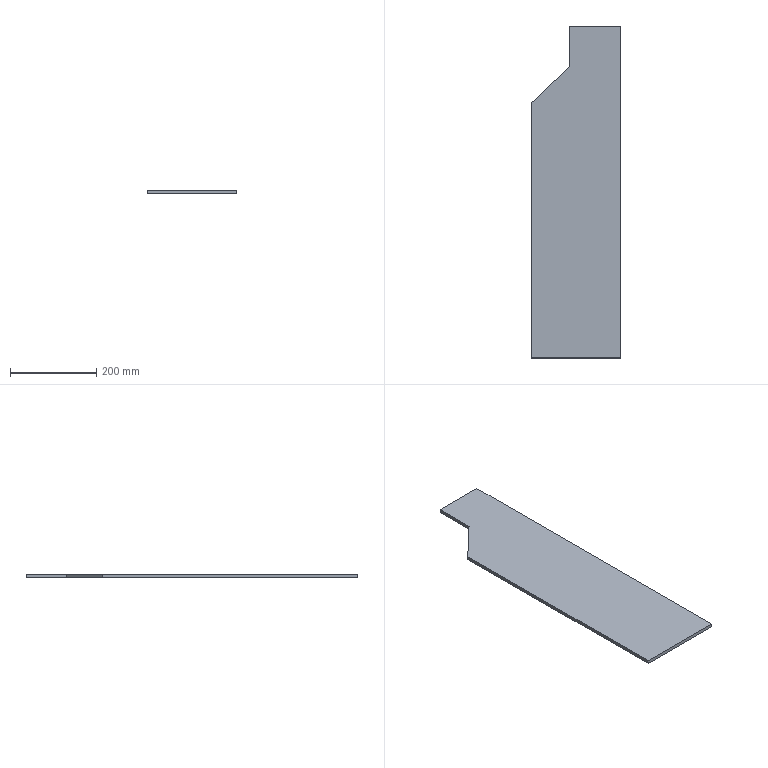Part | STEP file | Part 8 | 1 solid | 8 faces | box 208 x 768 x 8 mm | volume 1182208 mm3 | plane 8
STEP:
#1=CARTESIAN_POINT('',(0.,0.,0.));
#2=DIRECTION('',(0.,0.,1.));
#3=DIRECTION('',(1.,0.,0.));
#4=AXIS2_PLACEMENT_3D('',#1,#2,#3);
#5=CARTESIAN_POINT('',(0.,-384.,0.));
#6=VERTEX_POINT('',#5);
#7=CARTESIAN_POINT('',(0.,384.,0.));
#8=VERTEX_POINT('',#7);
#9=CARTESIAN_POINT('',(0.,-384.,0.));
#10=DIRECTION('',(0.,1.,0.));
#11=VECTOR('',#10,1.);
#12=LINE('',#9,#11);
#13=CARTESIAN_POINT('',(0.,-384.,8.));
#14=DIRECTION('',(-1.,0.,0.));
#15=DIRECTION('',(0.,0.,1.));
#16=AXIS2_PLACEMENT_3D('',#13,#14,#15);
#17=PLANE('',#16);
#18=CARTESIAN_POINT('',(-8.,0.));
#19=DIRECTION('',(0.,1.));
#20=VECTOR('',#19,1.);
#21=LINE('',#18,#20);
#22=(GEOMETRIC_REPRESENTATION_CONTEXT(2)PARAMETRIC_REPRESENTATION_CONTEXT()REPRESENTATION_CONTEXT('',''));
#23=DEFINITIONAL_REPRESENTATION('',(#21),#22);
#24=PCURVE('',#17,#23);
#25=CARTESIAN_POINT('',(0.,0.,0.));
#26=DIRECTION('',(0.,0.,-1.));
#27=DIRECTION('',(-1.,0.,0.));
#28=AXIS2_PLACEMENT_3D('',#25,#26,#27);
#29=PLANE('',#28);
#30=CARTESIAN_POINT('',(0.,-384.));
#31=DIRECTION('',(0.,1.));
#32=VECTOR('',#31,1.);
#33=LINE('',#30,#32);
#34=(GEOMETRIC_REPRESENTATION_CONTEXT(2)PARAMETRIC_REPRESENTATION_CONTEXT()REPRESENTATION_CONTEXT('',''));
#35=DEFINITIONAL_REPRESENTATION('',(#33),#34);
#36=PCURVE('',#29,#35);
#37=SURFACE_CURVE('',#12,(#24,#36),.PCURVE_S1.);
#38=EDGE_CURVE('',#6,#8,#37,.T.);
#39=ORIENTED_EDGE('',*,*,#38,.T.);
#40=CARTESIAN_POINT('',(0.,384.,8.));
#41=VERTEX_POINT('',#40);
#42=CARTESIAN_POINT('',(0.,384.,8.));
#43=DIRECTION('',(0.,0.,-1.));
#44=VECTOR('',#43,1.);
#45=LINE('',#42,#44);
#46=CARTESIAN_POINT('',(0.,768.));
#47=DIRECTION('',(-1.,0.));
#48=VECTOR('',#47,1.);
#49=LINE('',#46,#48);
#50=(GEOMETRIC_REPRESENTATION_CONTEXT(2)PARAMETRIC_REPRESENTATION_CONTEXT()REPRESENTATION_CONTEXT('',''));
#51=DEFINITIONAL_REPRESENTATION('',(#49),#50);
#52=PCURVE('',#17,#51);
#53=CARTESIAN_POINT('',(-120.,384.,8.));
#54=DIRECTION('',(0.,-1.,0.));
#55=DIRECTION('',(0.,0.,-1.));
#56=AXIS2_PLACEMENT_3D('',#53,#54,#55);
#57=PLANE('',#56);
#58=CARTESIAN_POINT('',(0.,120.));
#59=DIRECTION('',(1.,0.));
#60=VECTOR('',#59,1.);
#61=LINE('',#58,#60);
#62=(GEOMETRIC_REPRESENTATION_CONTEXT(2)PARAMETRIC_REPRESENTATION_CONTEXT()REPRESENTATION_CONTEXT('',''));
#63=DEFINITIONAL_REPRESENTATION('',(#61),#62);
#64=PCURVE('',#57,#63);
#65=SURFACE_CURVE('',#45,(#52,#64),.PCURVE_S1.);
#66=EDGE_CURVE('',#41,#8,#65,.T.);
#67=ORIENTED_EDGE('',*,*,#66,.F.);
#68=CARTESIAN_POINT('',(0.,-384.,8.));
#69=VERTEX_POINT('',#68);
#70=CARTESIAN_POINT('',(0.,-384.,8.));
#71=DIRECTION('',(0.,1.,0.));
#72=VECTOR('',#71,1.);
#73=LINE('',#70,#72);
#74=CARTESIAN_POINT('',(0.,0.));
#75=DIRECTION('',(0.,1.));
#76=VECTOR('',#75,1.);
#77=LINE('',#74,#76);
#78=(GEOMETRIC_REPRESENTATION_CONTEXT(2)PARAMETRIC_REPRESENTATION_CONTEXT()REPRESENTATION_CONTEXT('',''));
#79=DEFINITIONAL_REPRESENTATION('',(#77),#78);
#80=PCURVE('',#17,#79);
#81=CARTESIAN_POINT('',(0.,0.,8.));
#82=DIRECTION('',(0.,0.,-1.));
#83=DIRECTION('',(-1.,0.,0.));
#84=AXIS2_PLACEMENT_3D('',#81,#82,#83);
#85=PLANE('',#84);
#86=CARTESIAN_POINT('',(0.,-384.));
#87=DIRECTION('',(0.,1.));
#88=VECTOR('',#87,1.);
#89=LINE('',#86,#88);
#90=(GEOMETRIC_REPRESENTATION_CONTEXT(2)PARAMETRIC_REPRESENTATION_CONTEXT()REPRESENTATION_CONTEXT('',''));
#91=DEFINITIONAL_REPRESENTATION('',(#89),#90);
#92=PCURVE('',#85,#91);
#93=SURFACE_CURVE('',#73,(#80,#92),.PCURVE_S1.);
#94=EDGE_CURVE('',#69,#41,#93,.T.);
#95=ORIENTED_EDGE('',*,*,#94,.F.);
#96=CARTESIAN_POINT('',(0.,-384.,8.));
#97=DIRECTION('',(0.,0.,-1.));
#98=VECTOR('',#97,1.);
#99=LINE('',#96,#98);
#100=CARTESIAN_POINT('',(0.,0.));
#101=DIRECTION('',(-1.,0.));
#102=VECTOR('',#101,1.);
#103=LINE('',#100,#102);
#104=(GEOMETRIC_REPRESENTATION_CONTEXT(2)PARAMETRIC_REPRESENTATION_CONTEXT()REPRESENTATION_CONTEXT('',''));
#105=DEFINITIONAL_REPRESENTATION('',(#103),#104);
#106=PCURVE('',#17,#105);
#107=CARTESIAN_POINT('',(0.,-384.,8.));
#108=DIRECTION('',(0.,1.,0.));
#109=DIRECTION('',(0.,0.,1.));
#110=AXIS2_PLACEMENT_3D('',#107,#108,#109);
#111=PLANE('',#110);
#112=CARTESIAN_POINT('',(0.,0.));
#113=DIRECTION('',(-1.,0.));
#114=VECTOR('',#113,1.);
#115=LINE('',#112,#114);
#116=(GEOMETRIC_REPRESENTATION_CONTEXT(2)PARAMETRIC_REPRESENTATION_CONTEXT()REPRESENTATION_CONTEXT('',''));
#117=DEFINITIONAL_REPRESENTATION('',(#115),#116);
#118=PCURVE('',#111,#117);
#119=SURFACE_CURVE('',#99,(#106,#118),.PCURVE_S1.);
#120=EDGE_CURVE('',#69,#6,#119,.T.);
#121=ORIENTED_EDGE('',*,*,#120,.T.);
#122=EDGE_LOOP('',(#39,#67,#95,#121));
#123=FACE_BOUND('',#122,.T.);
#124=ADVANCED_FACE('',(#123),#17,.F.);
#125=CARTESIAN_POINT('',(-120.,384.,0.));
#126=VERTEX_POINT('',#125);
#127=CARTESIAN_POINT('',(-120.,384.,0.));
#128=DIRECTION('',(-1.,0.,0.));
#129=VECTOR('',#128,1.);
#130=LINE('',#127,#129);
#131=CARTESIAN_POINT('',(8.,0.));
#132=DIRECTION('',(0.,-1.));
#133=VECTOR('',#132,1.);
#134=LINE('',#131,#133);
#135=(GEOMETRIC_REPRESENTATION_CONTEXT(2)PARAMETRIC_REPRESENTATION_CONTEXT()REPRESENTATION_CONTEXT('',''));
#136=DEFINITIONAL_REPRESENTATION('',(#134),#135);
#137=PCURVE('',#57,#136);
#138=CARTESIAN_POINT('',(120.,384.));
#139=DIRECTION('',(1.,0.));
#140=VECTOR('',#139,1.);
#141=LINE('',#138,#140);
#142=(GEOMETRIC_REPRESENTATION_CONTEXT(2)PARAMETRIC_REPRESENTATION_CONTEXT()REPRESENTATION_CONTEXT('',''));
#143=DEFINITIONAL_REPRESENTATION('',(#141),#142);
#144=PCURVE('',#29,#143);
#145=SURFACE_CURVE('',#130,(#137,#144),.PCURVE_S1.);
#146=EDGE_CURVE('',#8,#126,#145,.T.);
#147=ORIENTED_EDGE('',*,*,#146,.T.);
#148=CARTESIAN_POINT('',(-120.,384.,8.));
#149=VERTEX_POINT('',#148);
#150=CARTESIAN_POINT('',(-120.,384.,8.));
#151=DIRECTION('',(0.,0.,-1.));
#152=VECTOR('',#151,1.);
#153=LINE('',#150,#152);
#154=CARTESIAN_POINT('',(0.,0.));
#155=DIRECTION('',(1.,0.));
#156=VECTOR('',#155,1.);
#157=LINE('',#154,#156);
#158=(GEOMETRIC_REPRESENTATION_CONTEXT(2)PARAMETRIC_REPRESENTATION_CONTEXT()REPRESENTATION_CONTEXT('',''));
#159=DEFINITIONAL_REPRESENTATION('',(#157),#158);
#160=PCURVE('',#57,#159);
#161=CARTESIAN_POINT('',(-120.,290.,8.));
#162=DIRECTION('',(1.,0.,0.));
#163=DIRECTION('',(0.,1.,0.));
#164=AXIS2_PLACEMENT_3D('',#161,#162,#163);
#165=PLANE('',#164);
#166=CARTESIAN_POINT('',(94.,0.));
#167=DIRECTION('',(0.,-1.));
#168=VECTOR('',#167,1.);
#169=LINE('',#166,#168);
#170=(GEOMETRIC_REPRESENTATION_CONTEXT(2)PARAMETRIC_REPRESENTATION_CONTEXT()REPRESENTATION_CONTEXT('',''));
#171=DEFINITIONAL_REPRESENTATION('',(#169),#170);
#172=PCURVE('',#165,#171);
#173=SURFACE_CURVE('',#153,(#160,#172),.PCURVE_S1.);
#174=EDGE_CURVE('',#149,#126,#173,.T.);
#175=ORIENTED_EDGE('',*,*,#174,.F.);
#176=CARTESIAN_POINT('',(-120.,384.,8.));
#177=DIRECTION('',(-1.,0.,0.));
#178=VECTOR('',#177,1.);
#179=LINE('',#176,#178);
#180=CARTESIAN_POINT('',(0.,0.));
#181=DIRECTION('',(0.,-1.));
#182=VECTOR('',#181,1.);
#183=LINE('',#180,#182);
#184=(GEOMETRIC_REPRESENTATION_CONTEXT(2)PARAMETRIC_REPRESENTATION_CONTEXT()REPRESENTATION_CONTEXT('',''));
#185=DEFINITIONAL_REPRESENTATION('',(#183),#184);
#186=PCURVE('',#57,#185);
#187=CARTESIAN_POINT('',(120.,384.));
#188=DIRECTION('',(1.,0.));
#189=VECTOR('',#188,1.);
#190=LINE('',#187,#189);
#191=(GEOMETRIC_REPRESENTATION_CONTEXT(2)PARAMETRIC_REPRESENTATION_CONTEXT()REPRESENTATION_CONTEXT('',''));
#192=DEFINITIONAL_REPRESENTATION('',(#190),#191);
#193=PCURVE('',#85,#192);
#194=SURFACE_CURVE('',#179,(#186,#193),.PCURVE_S1.);
#195=EDGE_CURVE('',#41,#149,#194,.T.);
#196=ORIENTED_EDGE('',*,*,#195,.F.);
#197=ORIENTED_EDGE('',*,*,#66,.T.);
#198=EDGE_LOOP('',(#147,#175,#196,#197));
#199=FACE_BOUND('',#198,.T.);
#200=ADVANCED_FACE('',(#199),#57,.F.);
#201=CARTESIAN_POINT('',(-120.,290.,0.));
#202=VERTEX_POINT('',#201);
#203=CARTESIAN_POINT('',(-120.,290.,0.));
#204=DIRECTION('',(0.,-1.,0.));
#205=VECTOR('',#204,1.);
#206=LINE('',#203,#205);
#207=CARTESIAN_POINT('',(0.,-8.));
#208=DIRECTION('',(-1.,0.));
#209=VECTOR('',#208,1.);
#210=LINE('',#207,#209);
#211=(GEOMETRIC_REPRESENTATION_CONTEXT(2)PARAMETRIC_REPRESENTATION_CONTEXT()REPRESENTATION_CONTEXT('',''));
#212=DEFINITIONAL_REPRESENTATION('',(#210),#211);
#213=PCURVE('',#165,#212);
#214=CARTESIAN_POINT('',(120.,290.));
#215=DIRECTION('',(0.,-1.));
#216=VECTOR('',#215,1.);
#217=LINE('',#214,#216);
#218=(GEOMETRIC_REPRESENTATION_CONTEXT(2)PARAMETRIC_REPRESENTATION_CONTEXT()REPRESENTATION_CONTEXT('',''));
#219=DEFINITIONAL_REPRESENTATION('',(#217),#218);
#220=PCURVE('',#29,#219);
#221=SURFACE_CURVE('',#206,(#213,#220),.PCURVE_S1.);
#222=EDGE_CURVE('',#126,#202,#221,.T.);
#223=ORIENTED_EDGE('',*,*,#222,.T.);
#224=CARTESIAN_POINT('',(-120.,290.,8.));
#225=VERTEX_POINT('',#224);
#226=CARTESIAN_POINT('',(-120.,290.,8.));
#227=DIRECTION('',(0.,0.,-1.));
#228=VECTOR('',#227,1.);
#229=LINE('',#226,#228);
#230=CARTESIAN_POINT('',(0.,0.));
#231=DIRECTION('',(0.,-1.));
#232=VECTOR('',#231,1.);
#233=LINE('',#230,#232);
#234=(GEOMETRIC_REPRESENTATION_CONTEXT(2)PARAMETRIC_REPRESENTATION_CONTEXT()REPRESENTATION_CONTEXT('',''));
#235=DEFINITIONAL_REPRESENTATION('',(#233),#234);
#236=PCURVE('',#165,#235);
#237=CARTESIAN_POINT('',(-208.,206.,8.));
#238=DIRECTION('',(0.6905,-0.7234,0.));
#239=DIRECTION('',(0.7234,0.6905,0.));
#240=AXIS2_PLACEMENT_3D('',#237,#238,#239);
#241=PLANE('',#240);
#242=CARTESIAN_POINT('',(121.655,0.));
#243=DIRECTION('',(0.,-1.));
#244=VECTOR('',#243,1.);
#245=LINE('',#242,#244);
#246=(GEOMETRIC_REPRESENTATION_CONTEXT(2)PARAMETRIC_REPRESENTATION_CONTEXT()REPRESENTATION_CONTEXT('',''));
#247=DEFINITIONAL_REPRESENTATION('',(#245),#246);
#248=PCURVE('',#241,#247);
#249=SURFACE_CURVE('',#229,(#236,#248),.PCURVE_S1.);
#250=EDGE_CURVE('',#225,#202,#249,.T.);
#251=ORIENTED_EDGE('',*,*,#250,.F.);
#252=CARTESIAN_POINT('',(-120.,290.,8.));
#253=DIRECTION('',(0.,-1.,0.));
#254=VECTOR('',#253,1.);
#255=LINE('',#252,#254);
#256=CARTESIAN_POINT('',(0.,0.));
#257=DIRECTION('',(-1.,0.));
#258=VECTOR('',#257,1.);
#259=LINE('',#256,#258);
#260=(GEOMETRIC_REPRESENTATION_CONTEXT(2)PARAMETRIC_REPRESENTATION_CONTEXT()REPRESENTATION_CONTEXT('',''));
#261=DEFINITIONAL_REPRESENTATION('',(#259),#260);
#262=PCURVE('',#165,#261);
#263=CARTESIAN_POINT('',(120.,290.));
#264=DIRECTION('',(0.,-1.));
#265=VECTOR('',#264,1.);
#266=LINE('',#263,#265);
#267=(GEOMETRIC_REPRESENTATION_CONTEXT(2)PARAMETRIC_REPRESENTATION_CONTEXT()REPRESENTATION_CONTEXT('',''));
#268=DEFINITIONAL_REPRESENTATION('',(#266),#267);
#269=PCURVE('',#85,#268);
#270=SURFACE_CURVE('',#255,(#262,#269),.PCURVE_S1.);
#271=EDGE_CURVE('',#149,#225,#270,.T.);
#272=ORIENTED_EDGE('',*,*,#271,.F.);
#273=ORIENTED_EDGE('',*,*,#174,.T.);
#274=EDGE_LOOP('',(#223,#251,#272,#273));
#275=FACE_BOUND('',#274,.T.);
#276=ADVANCED_FACE('',(#275),#165,.F.);
#277=CARTESIAN_POINT('',(-208.,206.,0.));
#278=VERTEX_POINT('',#277);
#279=CARTESIAN_POINT('',(-208.,206.,0.));
#280=DIRECTION('',(-0.7234,-0.6905,0.));
#281=VECTOR('',#280,1.);
#282=LINE('',#279,#281);
#283=CARTESIAN_POINT('',(0.,-8.));
#284=DIRECTION('',(-1.,0.));
#285=VECTOR('',#284,1.);
#286=LINE('',#283,#285);
#287=(GEOMETRIC_REPRESENTATION_CONTEXT(2)PARAMETRIC_REPRESENTATION_CONTEXT()REPRESENTATION_CONTEXT('',''));
#288=DEFINITIONAL_REPRESENTATION('',(#286),#287);
#289=PCURVE('',#241,#288);
#290=CARTESIAN_POINT('',(208.,206.));
#291=DIRECTION('',(0.7234,-0.6905));
#292=VECTOR('',#291,1.);
#293=LINE('',#290,#292);
#294=(GEOMETRIC_REPRESENTATION_CONTEXT(2)PARAMETRIC_REPRESENTATION_CONTEXT()REPRESENTATION_CONTEXT('',''));
#295=DEFINITIONAL_REPRESENTATION('',(#293),#294);
#296=PCURVE('',#29,#295);
#297=SURFACE_CURVE('',#282,(#289,#296),.PCURVE_S1.);
#298=EDGE_CURVE('',#202,#278,#297,.T.);
#299=ORIENTED_EDGE('',*,*,#298,.T.);
#300=CARTESIAN_POINT('',(-208.,206.,8.));
#301=VERTEX_POINT('',#300);
#302=CARTESIAN_POINT('',(-208.,206.,8.));
#303=DIRECTION('',(0.,0.,-1.));
#304=VECTOR('',#303,1.);
#305=LINE('',#302,#304);
#306=CARTESIAN_POINT('',(0.,0.));
#307=DIRECTION('',(0.,-1.));
#308=VECTOR('',#307,1.);
#309=LINE('',#306,#308);
#310=(GEOMETRIC_REPRESENTATION_CONTEXT(2)PARAMETRIC_REPRESENTATION_CONTEXT()REPRESENTATION_CONTEXT('',''));
#311=DEFINITIONAL_REPRESENTATION('',(#309),#310);
#312=PCURVE('',#241,#311);
#313=CARTESIAN_POINT('',(-208.,-384.,8.));
#314=DIRECTION('',(1.,0.,0.));
#315=DIRECTION('',(0.,0.,-1.));
#316=AXIS2_PLACEMENT_3D('',#313,#314,#315);
#317=PLANE('',#316);
#318=CARTESIAN_POINT('',(0.,590.));
#319=DIRECTION('',(1.,0.));
#320=VECTOR('',#319,1.);
#321=LINE('',#318,#320);
#322=(GEOMETRIC_REPRESENTATION_CONTEXT(2)PARAMETRIC_REPRESENTATION_CONTEXT()REPRESENTATION_CONTEXT('',''));
#323=DEFINITIONAL_REPRESENTATION('',(#321),#322);
#324=PCURVE('',#317,#323);
#325=SURFACE_CURVE('',#305,(#312,#324),.PCURVE_S1.);
#326=EDGE_CURVE('',#301,#278,#325,.T.);
#327=ORIENTED_EDGE('',*,*,#326,.F.);
#328=CARTESIAN_POINT('',(-208.,206.,8.));
#329=DIRECTION('',(-0.7234,-0.6905,0.));
#330=VECTOR('',#329,1.);
#331=LINE('',#328,#330);
#332=CARTESIAN_POINT('',(0.,0.));
#333=DIRECTION('',(-1.,0.));
#334=VECTOR('',#333,1.);
#335=LINE('',#332,#334);
#336=(GEOMETRIC_REPRESENTATION_CONTEXT(2)PARAMETRIC_REPRESENTATION_CONTEXT()REPRESENTATION_CONTEXT('',''));
#337=DEFINITIONAL_REPRESENTATION('',(#335),#336);
#338=PCURVE('',#241,#337);
#339=CARTESIAN_POINT('',(208.,206.));
#340=DIRECTION('',(0.7234,-0.6905));
#341=VECTOR('',#340,1.);
#342=LINE('',#339,#341);
#343=(GEOMETRIC_REPRESENTATION_CONTEXT(2)PARAMETRIC_REPRESENTATION_CONTEXT()REPRESENTATION_CONTEXT('',''));
#344=DEFINITIONAL_REPRESENTATION('',(#342),#343);
#345=PCURVE('',#85,#344);
#346=SURFACE_CURVE('',#331,(#338,#345),.PCURVE_S1.);
#347=EDGE_CURVE('',#225,#301,#346,.T.);
#348=ORIENTED_EDGE('',*,*,#347,.F.);
#349=ORIENTED_EDGE('',*,*,#250,.T.);
#350=EDGE_LOOP('',(#299,#327,#348,#349));
#351=FACE_BOUND('',#350,.T.);
#352=ADVANCED_FACE('',(#351),#241,.F.);
#353=CARTESIAN_POINT('',(-208.,-384.,0.));
#354=VERTEX_POINT('',#353);
#355=CARTESIAN_POINT('',(-208.,-384.,0.));
#356=DIRECTION('',(0.,-1.,0.));
#357=VECTOR('',#356,1.);
#358=LINE('',#355,#357);
#359=CARTESIAN_POINT('',(8.,0.));
#360=DIRECTION('',(0.,-1.));
#361=VECTOR('',#360,1.);
#362=LINE('',#359,#361);
#363=(GEOMETRIC_REPRESENTATION_CONTEXT(2)PARAMETRIC_REPRESENTATION_CONTEXT()REPRESENTATION_CONTEXT('',''));
#364=DEFINITIONAL_REPRESENTATION('',(#362),#363);
#365=PCURVE('',#317,#364);
#366=CARTESIAN_POINT('',(208.,-384.));
#367=DIRECTION('',(0.,-1.));
#368=VECTOR('',#367,1.);
#369=LINE('',#366,#368);
#370=(GEOMETRIC_REPRESENTATION_CONTEXT(2)PARAMETRIC_REPRESENTATION_CONTEXT()REPRESENTATION_CONTEXT('',''));
#371=DEFINITIONAL_REPRESENTATION('',(#369),#370);
#372=PCURVE('',#29,#371);
#373=SURFACE_CURVE('',#358,(#365,#372),.PCURVE_S1.);
#374=EDGE_CURVE('',#278,#354,#373,.T.);
#375=ORIENTED_EDGE('',*,*,#374,.T.);
#376=CARTESIAN_POINT('',(-208.,-384.,8.));
#377=VERTEX_POINT('',#376);
#378=CARTESIAN_POINT('',(-208.,-384.,8.));
#379=DIRECTION('',(0.,0.,-1.));
#380=VECTOR('',#379,1.);
#381=LINE('',#378,#380);
#382=CARTESIAN_POINT('',(0.,0.));
#383=DIRECTION('',(1.,0.));
#384=VECTOR('',#383,1.);
#385=LINE('',#382,#384);
#386=(GEOMETRIC_REPRESENTATION_CONTEXT(2)PARAMETRIC_REPRESENTATION_CONTEXT()REPRESENTATION_CONTEXT('',''));
#387=DEFINITIONAL_REPRESENTATION('',(#385),#386);
#388=PCURVE('',#317,#387);
#389=CARTESIAN_POINT('',(0.,-208.));
#390=DIRECTION('',(-1.,0.));
#391=VECTOR('',#390,1.);
#392=LINE('',#389,#391);
#393=(GEOMETRIC_REPRESENTATION_CONTEXT(2)PARAMETRIC_REPRESENTATION_CONTEXT()REPRESENTATION_CONTEXT('',''));
#394=DEFINITIONAL_REPRESENTATION('',(#392),#393);
#395=PCURVE('',#111,#394);
#396=SURFACE_CURVE('',#381,(#388,#395),.PCURVE_S1.);
#397=EDGE_CURVE('',#377,#354,#396,.T.);
#398=ORIENTED_EDGE('',*,*,#397,.F.);
#399=CARTESIAN_POINT('',(-208.,-384.,8.));
#400=DIRECTION('',(0.,-1.,0.));
#401=VECTOR('',#400,1.);
#402=LINE('',#399,#401);
#403=CARTESIAN_POINT('',(0.,0.));
#404=DIRECTION('',(0.,-1.));
#405=VECTOR('',#404,1.);
#406=LINE('',#403,#405);
#407=(GEOMETRIC_REPRESENTATION_CONTEXT(2)PARAMETRIC_REPRESENTATION_CONTEXT()REPRESENTATION_CONTEXT('',''));
#408=DEFINITIONAL_REPRESENTATION('',(#406),#407);
#409=PCURVE('',#317,#408);
#410=CARTESIAN_POINT('',(208.,-384.));
#411=DIRECTION('',(0.,-1.));
#412=VECTOR('',#411,1.);
#413=LINE('',#410,#412);
#414=(GEOMETRIC_REPRESENTATION_CONTEXT(2)PARAMETRIC_REPRESENTATION_CONTEXT()REPRESENTATION_CONTEXT('',''));
#415=DEFINITIONAL_REPRESENTATION('',(#413),#414);
#416=PCURVE('',#85,#415);
#417=SURFACE_CURVE('',#402,(#409,#416),.PCURVE_S1.);
#418=EDGE_CURVE('',#301,#377,#417,.T.);
#419=ORIENTED_EDGE('',*,*,#418,.F.);
#420=ORIENTED_EDGE('',*,*,#326,.T.);
#421=EDGE_LOOP('',(#375,#398,#419,#420));
#422=FACE_BOUND('',#421,.T.);
#423=ADVANCED_FACE('',(#422),#317,.F.);
#424=CARTESIAN_POINT('',(0.,-384.,0.));
#425=DIRECTION('',(1.,0.,0.));
#426=VECTOR('',#425,1.);
#427=LINE('',#424,#426);
#428=CARTESIAN_POINT('',(-8.,0.));
#429=DIRECTION('',(0.,1.));
#430=VECTOR('',#429,1.);
#431=LINE('',#428,#430);
#432=(GEOMETRIC_REPRESENTATION_CONTEXT(2)PARAMETRIC_REPRESENTATION_CONTEXT()REPRESENTATION_CONTEXT('',''));
#433=DEFINITIONAL_REPRESENTATION('',(#431),#432);
#434=PCURVE('',#111,#433);
#435=CARTESIAN_POINT('',(0.,-384.));
#436=DIRECTION('',(-1.,0.));
#437=VECTOR('',#436,1.);
#438=LINE('',#435,#437);
#439=(GEOMETRIC_REPRESENTATION_CONTEXT(2)PARAMETRIC_REPRESENTATION_CONTEXT()REPRESENTATION_CONTEXT('',''));
#440=DEFINITIONAL_REPRESENTATION('',(#438),#439);
#441=PCURVE('',#29,#440);
#442=SURFACE_CURVE('',#427,(#434,#441),.PCURVE_S1.);
#443=EDGE_CURVE('',#354,#6,#442,.T.);
#444=ORIENTED_EDGE('',*,*,#443,.T.);
#445=ORIENTED_EDGE('',*,*,#120,.F.);
#446=CARTESIAN_POINT('',(0.,-384.,8.));
#447=DIRECTION('',(1.,0.,0.));
#448=VECTOR('',#447,1.);
#449=LINE('',#446,#448);
#450=CARTESIAN_POINT('',(0.,0.));
#451=DIRECTION('',(0.,1.));
#452=VECTOR('',#451,1.);
#453=LINE('',#450,#452);
#454=(GEOMETRIC_REPRESENTATION_CONTEXT(2)PARAMETRIC_REPRESENTATION_CONTEXT()REPRESENTATION_CONTEXT('',''));
#455=DEFINITIONAL_REPRESENTATION('',(#453),#454);
#456=PCURVE('',#111,#455);
#457=CARTESIAN_POINT('',(0.,-384.));
#458=DIRECTION('',(-1.,0.));
#459=VECTOR('',#458,1.);
#460=LINE('',#457,#459);
#461=(GEOMETRIC_REPRESENTATION_CONTEXT(2)PARAMETRIC_REPRESENTATION_CONTEXT()REPRESENTATION_CONTEXT('',''));
#462=DEFINITIONAL_REPRESENTATION('',(#460),#461);
#463=PCURVE('',#85,#462);
#464=SURFACE_CURVE('',#449,(#456,#463),.PCURVE_S1.);
#465=EDGE_CURVE('',#377,#69,#464,.T.);
#466=ORIENTED_EDGE('',*,*,#465,.F.);
#467=ORIENTED_EDGE('',*,*,#397,.T.);
#468=EDGE_LOOP('',(#444,#445,#466,#467));
#469=FACE_BOUND('',#468,.T.);
#470=ADVANCED_FACE('',(#469),#111,.F.);
#471=ORIENTED_EDGE('',*,*,#94,.T.);
#472=ORIENTED_EDGE('',*,*,#195,.T.);
#473=ORIENTED_EDGE('',*,*,#271,.T.);
#474=ORIENTED_EDGE('',*,*,#347,.T.);
#475=ORIENTED_EDGE('',*,*,#418,.T.);
#476=ORIENTED_EDGE('',*,*,#465,.T.);
#477=EDGE_LOOP('',(#471,#472,#473,#474,#475,#476));
#478=FACE_BOUND('',#477,.T.);
#479=ADVANCED_FACE('',(#478),#85,.F.);
#480=ORIENTED_EDGE('',*,*,#38,.F.);
#481=ORIENTED_EDGE('',*,*,#443,.F.);
#482=ORIENTED_EDGE('',*,*,#374,.F.);
#483=ORIENTED_EDGE('',*,*,#298,.F.);
#484=ORIENTED_EDGE('',*,*,#222,.F.);
#485=ORIENTED_EDGE('',*,*,#146,.F.);
#486=EDGE_LOOP('',(#480,#481,#482,#483,#484,#485));
#487=FACE_BOUND('',#486,.T.);
#488=ADVANCED_FACE('',(#487),#29,.T.);
#489=CLOSED_SHELL('',(#124,#200,#276,#352,#423,#470,#479,#488));
#490=MANIFOLD_SOLID_BREP('',#489);
#491=(LENGTH_UNIT()NAMED_UNIT(*)SI_UNIT(.MILLI.,.METRE.));
#492=UNCERTAINTY_MEASURE_WITH_UNIT(LENGTH_MEASURE(0.0000001),#491,'','');
#493=(NAMED_UNIT(*)PLANE_ANGLE_UNIT()SI_UNIT($,.RADIAN.));
#494=(NAMED_UNIT(*)SI_UNIT($,.STERADIAN.)SOLID_ANGLE_UNIT());
#495=(GEOMETRIC_REPRESENTATION_CONTEXT(3)GLOBAL_UNCERTAINTY_ASSIGNED_CONTEXT((#492))GLOBAL_UNIT_ASSIGNED_CONTEXT((#491,#493,#494))REPRESENTATION_CONTEXT('',''));
#496=ADVANCED_BREP_SHAPE_REPRESENTATION('',(#4,#490),#495);